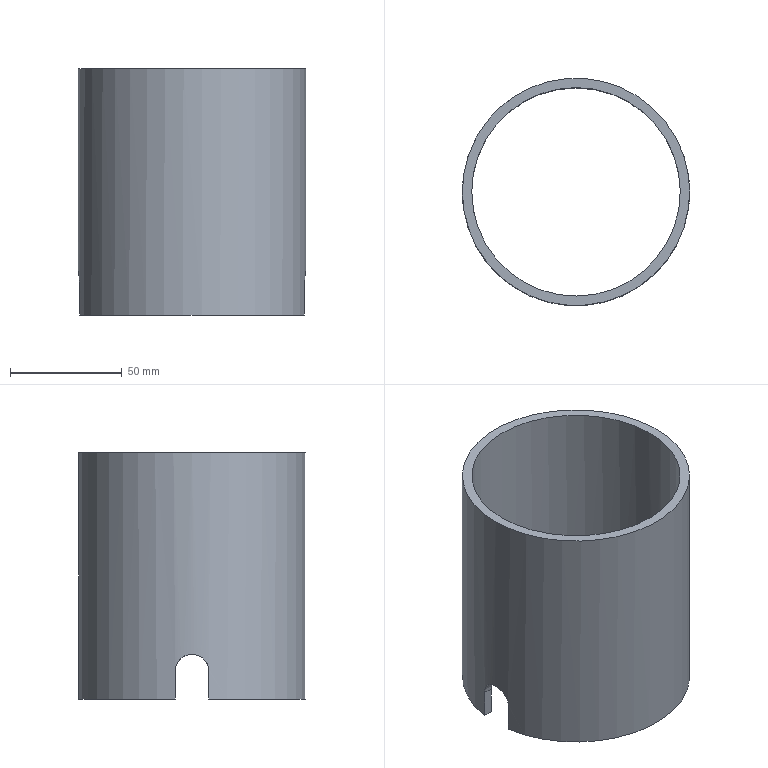Part | NX | features solid 2 | 1 solid | 11 faces | box 101.6 x 101.6 x 110 mm | volume 139042 mm3 | plane 7 | cylinder 4 | commonest cylinder face diameters 15 x2 93.2 x1 101.6 x1
STEP:
#1=CARTESIAN_POINT('',(-1250.243,532.5,-195.));
#2=VERTEX_POINT('',#1);
#3=CARTESIAN_POINT('',(-1245.992,532.5,-195.));
#4=VERTEX_POINT('',#3);
#5=CARTESIAN_POINT('',(-1200.,532.5,-195.));
#6=DIRECTION('',(1.,0.,0.));
#7=VECTOR('',#6,1000.);
#8=LINE('',#5,#7);
#9=EDGE_CURVE('',#2,#4,#8,.T.);
#10=ORIENTED_EDGE('',*,*,#9,.F.);
#11=CARTESIAN_POINT('',(-1149.757,532.5,-195.));
#12=VERTEX_POINT('',#11);
#13=CARTESIAN_POINT('',(-1200.,525.,-195.));
#14=DIRECTION('',(0.,0.,1.));
#15=DIRECTION('',(-1.,0.,0.));
#16=AXIS2_PLACEMENT_3D('',#13,#14,#15);
#17=CIRCLE('',#16,50.8);
#18=EDGE_CURVE('',#12,#2,#17,.T.);
#19=ORIENTED_EDGE('',*,*,#18,.F.);
#20=CARTESIAN_POINT('',(-1154.008,532.5,-195.));
#21=VERTEX_POINT('',#20);
#22=CARTESIAN_POINT('',(-1130.25,532.5,-195.));
#23=DIRECTION('',(-1.,0.,0.));
#24=VECTOR('',#23,1000.);
#25=LINE('',#22,#24);
#26=EDGE_CURVE('',#12,#21,#25,.T.);
#27=ORIENTED_EDGE('',*,*,#26,.T.);
#28=CARTESIAN_POINT('',(-1200.,525.,-195.));
#29=DIRECTION('',(0.,0.,1.));
#30=DIRECTION('',(-1.,0.,0.));
#31=AXIS2_PLACEMENT_3D('',#28,#29,#30);
#32=CIRCLE('',#31,46.6);
#33=EDGE_CURVE('',#21,#4,#32,.T.);
#34=ORIENTED_EDGE('',*,*,#33,.T.);
#35=EDGE_LOOP('',(#10,#19,#27,#34));
#36=FACE_BOUND('',#35,.T.);
#37=CARTESIAN_POINT('',(-1200.,525.,-195.));
#38=DIRECTION('',(0.,0.,1.));
#39=DIRECTION('',(-1.,0.,0.));
#40=AXIS2_PLACEMENT_3D('',#37,#38,#39);
#41=PLANE('',#40);
#42=ADVANCED_FACE('',(#36),#41,.F.);
#43=CARTESIAN_POINT('',(-1250.243,517.5,-195.));
#44=VERTEX_POINT('',#43);
#45=CARTESIAN_POINT('',(-1149.757,517.5,-195.));
#46=VERTEX_POINT('',#45);
#47=CARTESIAN_POINT('',(-1200.,525.,-195.));
#48=DIRECTION('',(0.,0.,1.));
#49=DIRECTION('',(-1.,0.,0.));
#50=AXIS2_PLACEMENT_3D('',#47,#48,#49);
#51=CIRCLE('',#50,50.8);
#52=EDGE_CURVE('',#44,#46,#51,.T.);
#53=ORIENTED_EDGE('',*,*,#52,.T.);
#54=CARTESIAN_POINT('',(-1149.757,517.5,-182.5));
#55=VERTEX_POINT('',#54);
#56=CARTESIAN_POINT('',(-1149.757,517.5,-195.));
#57=DIRECTION('',(0.,0.,-1.));
#58=VECTOR('',#57,1000.);
#59=LINE('',#56,#58);
#60=EDGE_CURVE('',#46,#55,#59,.F.);
#61=ORIENTED_EDGE('',*,*,#60,.T.);
#62=CARTESIAN_POINT('',(-1149.757,532.5,-182.5));
#63=VERTEX_POINT('',#62);
#64=CARTESIAN_POINT('',(-1149.757,517.5,-182.5));
#65=CARTESIAN_POINT('',(-1149.757,517.5,-180.54));
#66=CARTESIAN_POINT('',(-1149.477,519.114,-176.63));
#67=CARTESIAN_POINT('',(-1149.061,525.012,-174.184));
#68=CARTESIAN_POINT('',(-1149.477,530.875,-176.636));
#69=CARTESIAN_POINT('',(-1149.757,532.5,-180.518));
#70=CARTESIAN_POINT('',(-1149.757,532.5,-182.5));
#71=B_SPLINE_CURVE_WITH_KNOTS('',3,(#64,#65,#66,#67,#68,#69,#70),.UNSPECIFIED.,.F.,.F.,(4,1,1,1,4),(0.03597,0.04184,0.04771,0.05358,0.05945),.UNSPECIFIED.);
#72=EDGE_CURVE('',#55,#63,#71,.T.);
#73=ORIENTED_EDGE('',*,*,#72,.T.);
#74=CARTESIAN_POINT('',(-1149.757,532.5,-135.));
#75=DIRECTION('',(0.,0.,-1.));
#76=VECTOR('',#75,1000.);
#77=LINE('',#74,#76);
#78=EDGE_CURVE('',#12,#63,#77,.F.);
#79=ORIENTED_EDGE('',*,*,#78,.F.);
#80=ORIENTED_EDGE('',*,*,#18,.T.);
#81=CARTESIAN_POINT('',(-1250.243,532.5,-182.5));
#82=VERTEX_POINT('',#81);
#83=CARTESIAN_POINT('',(-1250.243,532.5,-135.));
#84=DIRECTION('',(0.,0.,-1.));
#85=VECTOR('',#84,1000.);
#86=LINE('',#83,#85);
#87=EDGE_CURVE('',#82,#2,#86,.T.);
#88=ORIENTED_EDGE('',*,*,#87,.F.);
#89=CARTESIAN_POINT('',(-1250.243,517.5,-182.5));
#90=VERTEX_POINT('',#89);
#91=CARTESIAN_POINT('',(-1250.243,532.5,-182.5));
#92=CARTESIAN_POINT('',(-1250.243,532.5,-180.54));
#93=CARTESIAN_POINT('',(-1250.523,530.886,-176.63));
#94=CARTESIAN_POINT('',(-1250.939,524.988,-174.184));
#95=CARTESIAN_POINT('',(-1250.523,519.125,-176.636));
#96=CARTESIAN_POINT('',(-1250.243,517.5,-180.518));
#97=CARTESIAN_POINT('',(-1250.243,517.5,-182.5));
#98=B_SPLINE_CURVE_WITH_KNOTS('',3,(#91,#92,#93,#94,#95,#96,#97),.UNSPECIFIED.,.F.,.F.,(4,1,1,1,4),(0.03597,0.04184,0.04771,0.05358,0.05945),.UNSPECIFIED.);
#99=EDGE_CURVE('',#82,#90,#98,.T.);
#100=ORIENTED_EDGE('',*,*,#99,.T.);
#101=CARTESIAN_POINT('',(-1250.243,517.5,-135.));
#102=DIRECTION('',(0.,0.,-1.));
#103=VECTOR('',#102,1000.);
#104=LINE('',#101,#103);
#105=EDGE_CURVE('',#90,#44,#104,.T.);
#106=ORIENTED_EDGE('',*,*,#105,.T.);
#107=EDGE_LOOP('',(#53,#61,#73,#79,#80,#88,#100,#106));
#108=FACE_BOUND('',#107,.T.);
#109=CARTESIAN_POINT('',(-1250.8,525.,-85.));
#110=VERTEX_POINT('',#109);
#111=CARTESIAN_POINT('',(-1200.,525.,-85.));
#112=DIRECTION('',(0.,0.,1.));
#113=DIRECTION('',(-1.,0.,0.));
#114=AXIS2_PLACEMENT_3D('',#111,#112,#113);
#115=CIRCLE('',#114,50.8);
#116=EDGE_CURVE('',#110,#110,#115,.T.);
#117=ORIENTED_EDGE('',*,*,#116,.F.);
#118=EDGE_LOOP('',(#117));
#119=FACE_BOUND('',#118,.T.);
#120=CARTESIAN_POINT('',(-1200.,525.,-135.));
#121=DIRECTION('',(0.,0.,-1.));
#122=DIRECTION('',(1.,0.,0.));
#123=AXIS2_PLACEMENT_3D('',#120,#121,#122);
#124=CYLINDRICAL_SURFACE('',#123,50.8);
#125=ADVANCED_FACE('',(#108,#119),#124,.T.);
#126=CARTESIAN_POINT('',(-1154.008,517.5,-195.));
#127=VERTEX_POINT('',#126);
#128=CARTESIAN_POINT('',(-1154.008,517.5,-182.5));
#129=VERTEX_POINT('',#128);
#130=CARTESIAN_POINT('',(-1154.008,517.5,-135.));
#131=DIRECTION('',(0.,0.,-1.));
#132=VECTOR('',#131,1000.);
#133=LINE('',#130,#132);
#134=EDGE_CURVE('',#127,#129,#133,.F.);
#135=ORIENTED_EDGE('',*,*,#134,.F.);
#136=CARTESIAN_POINT('',(-1245.992,517.5,-195.));
#137=VERTEX_POINT('',#136);
#138=CARTESIAN_POINT('',(-1200.,525.,-195.));
#139=DIRECTION('',(0.,0.,1.));
#140=DIRECTION('',(-1.,0.,0.));
#141=AXIS2_PLACEMENT_3D('',#138,#139,#140);
#142=CIRCLE('',#141,46.6);
#143=EDGE_CURVE('',#137,#127,#142,.T.);
#144=ORIENTED_EDGE('',*,*,#143,.F.);
#145=CARTESIAN_POINT('',(-1245.992,517.5,-182.5));
#146=VERTEX_POINT('',#145);
#147=CARTESIAN_POINT('',(-1245.992,517.5,-135.));
#148=DIRECTION('',(0.,0.,-1.));
#149=VECTOR('',#148,1000.);
#150=LINE('',#147,#149);
#151=EDGE_CURVE('',#146,#137,#150,.T.);
#152=ORIENTED_EDGE('',*,*,#151,.F.);
#153=CARTESIAN_POINT('',(-1245.992,532.5,-182.5));
#154=VERTEX_POINT('',#153);
#155=CARTESIAN_POINT('',(-1245.992,532.5,-182.5));
#156=CARTESIAN_POINT('',(-1245.992,532.5,-180.542));
#157=CARTESIAN_POINT('',(-1246.298,530.886,-176.629));
#158=CARTESIAN_POINT('',(-1246.751,524.99,-174.184));
#159=CARTESIAN_POINT('',(-1246.298,519.126,-176.633));
#160=CARTESIAN_POINT('',(-1245.992,517.5,-180.52));
#161=CARTESIAN_POINT('',(-1245.992,517.5,-182.5));
#162=B_SPLINE_CURVE_WITH_KNOTS('',3,(#155,#156,#157,#158,#159,#160,#161),.UNSPECIFIED.,.F.,.F.,(4,1,1,1,4),(0.03615,0.04202,0.04789,0.05376,0.05963),.UNSPECIFIED.);
#163=EDGE_CURVE('',#154,#146,#162,.T.);
#164=ORIENTED_EDGE('',*,*,#163,.F.);
#165=CARTESIAN_POINT('',(-1245.992,532.5,-135.));
#166=DIRECTION('',(0.,0.,-1.));
#167=VECTOR('',#166,1000.);
#168=LINE('',#165,#167);
#169=EDGE_CURVE('',#154,#4,#168,.T.);
#170=ORIENTED_EDGE('',*,*,#169,.T.);
#171=ORIENTED_EDGE('',*,*,#33,.F.);
#172=CARTESIAN_POINT('',(-1154.008,532.5,-182.5));
#173=VERTEX_POINT('',#172);
#174=CARTESIAN_POINT('',(-1154.008,532.5,-135.));
#175=DIRECTION('',(0.,0.,-1.));
#176=VECTOR('',#175,1000.);
#177=LINE('',#174,#176);
#178=EDGE_CURVE('',#21,#173,#177,.F.);
#179=ORIENTED_EDGE('',*,*,#178,.T.);
#180=CARTESIAN_POINT('',(-1154.008,517.5,-182.5));
#181=CARTESIAN_POINT('',(-1154.008,517.5,-180.542));
#182=CARTESIAN_POINT('',(-1153.702,519.114,-176.629));
#183=CARTESIAN_POINT('',(-1153.249,525.01,-174.184));
#184=CARTESIAN_POINT('',(-1153.702,530.874,-176.633));
#185=CARTESIAN_POINT('',(-1154.008,532.5,-180.52));
#186=CARTESIAN_POINT('',(-1154.008,532.5,-182.5));
#187=B_SPLINE_CURVE_WITH_KNOTS('',3,(#180,#181,#182,#183,#184,#185,#186),.UNSPECIFIED.,.F.,.F.,(4,1,1,1,4),(0.03615,0.04202,0.04789,0.05376,0.05963),.UNSPECIFIED.);
#188=EDGE_CURVE('',#129,#173,#187,.T.);
#189=ORIENTED_EDGE('',*,*,#188,.F.);
#190=EDGE_LOOP('',(#135,#144,#152,#164,#170,#171,#179,#189));
#191=FACE_BOUND('',#190,.T.);
#192=CARTESIAN_POINT('',(-1246.6,525.,-85.));
#193=VERTEX_POINT('',#192);
#194=CARTESIAN_POINT('',(-1200.,525.,-85.));
#195=DIRECTION('',(0.,0.,1.));
#196=DIRECTION('',(-1.,0.,0.));
#197=AXIS2_PLACEMENT_3D('',#194,#195,#196);
#198=CIRCLE('',#197,46.6);
#199=EDGE_CURVE('',#193,#193,#198,.T.);
#200=ORIENTED_EDGE('',*,*,#199,.T.);
#201=EDGE_LOOP('',(#200));
#202=FACE_BOUND('',#201,.T.);
#203=CARTESIAN_POINT('',(-1200.,525.,-135.));
#204=DIRECTION('',(0.,0.,-1.));
#205=DIRECTION('',(1.,0.,0.));
#206=AXIS2_PLACEMENT_3D('',#203,#204,#205);
#207=CYLINDRICAL_SURFACE('',#206,46.6);
#208=ADVANCED_FACE('',(#191,#202),#207,.F.);
#209=ORIENTED_EDGE('',*,*,#116,.T.);
#210=EDGE_LOOP('',(#209));
#211=FACE_BOUND('',#210,.T.);
#212=ORIENTED_EDGE('',*,*,#199,.F.);
#213=EDGE_LOOP('',(#212));
#214=FACE_BOUND('',#213,.T.);
#215=CARTESIAN_POINT('',(-1200.,525.,-85.));
#216=DIRECTION('',(0.,0.,1.));
#217=DIRECTION('',(-1.,0.,0.));
#218=AXIS2_PLACEMENT_3D('',#215,#216,#217);
#219=PLANE('',#218);
#220=ADVANCED_FACE('',(#211,#214),#219,.T.);
#221=ORIENTED_EDGE('',*,*,#52,.F.);
#222=CARTESIAN_POINT('',(-1200.,517.5,-195.));
#223=DIRECTION('',(1.,0.,0.));
#224=VECTOR('',#223,1000.);
#225=LINE('',#222,#224);
#226=EDGE_CURVE('',#44,#137,#225,.T.);
#227=ORIENTED_EDGE('',*,*,#226,.T.);
#228=ORIENTED_EDGE('',*,*,#143,.T.);
#229=CARTESIAN_POINT('',(-1130.25,517.5,-195.));
#230=DIRECTION('',(-1.,0.,0.));
#231=VECTOR('',#230,1000.);
#232=LINE('',#229,#231);
#233=EDGE_CURVE('',#46,#127,#232,.T.);
#234=ORIENTED_EDGE('',*,*,#233,.F.);
#235=EDGE_LOOP('',(#221,#227,#228,#234));
#236=FACE_BOUND('',#235,.T.);
#237=CARTESIAN_POINT('',(-1200.,525.,-195.));
#238=DIRECTION('',(0.,0.,1.));
#239=DIRECTION('',(-1.,0.,0.));
#240=AXIS2_PLACEMENT_3D('',#237,#238,#239);
#241=PLANE('',#240);
#242=ADVANCED_FACE('',(#236),#241,.F.);
#243=ORIENTED_EDGE('',*,*,#78,.T.);
#244=CARTESIAN_POINT('',(-1130.25,532.5,-182.5));
#245=DIRECTION('',(-1.,0.,0.));
#246=VECTOR('',#245,1000.);
#247=LINE('',#244,#246);
#248=EDGE_CURVE('',#173,#63,#247,.F.);
#249=ORIENTED_EDGE('',*,*,#248,.F.);
#250=ORIENTED_EDGE('',*,*,#178,.F.);
#251=ORIENTED_EDGE('',*,*,#26,.F.);
#252=EDGE_LOOP('',(#243,#249,#250,#251));
#253=FACE_BOUND('',#252,.T.);
#254=CARTESIAN_POINT('',(-1130.25,532.5,-195.));
#255=DIRECTION('',(0.,-1.,0.));
#256=DIRECTION('',(0.,0.,1.));
#257=AXIS2_PLACEMENT_3D('',#254,#255,#256);
#258=PLANE('',#257);
#259=ADVANCED_FACE('',(#253),#258,.T.);
#260=ORIENTED_EDGE('',*,*,#233,.T.);
#261=ORIENTED_EDGE('',*,*,#134,.T.);
#262=CARTESIAN_POINT('',(-1330.25,517.5,-182.5));
#263=DIRECTION('',(-1.,0.,0.));
#264=VECTOR('',#263,1000.);
#265=LINE('',#262,#264);
#266=EDGE_CURVE('',#55,#129,#265,.T.);
#267=ORIENTED_EDGE('',*,*,#266,.F.);
#268=ORIENTED_EDGE('',*,*,#60,.F.);
#269=EDGE_LOOP('',(#260,#261,#267,#268));
#270=FACE_BOUND('',#269,.T.);
#271=CARTESIAN_POINT('',(-1130.25,517.5,-195.));
#272=DIRECTION('',(0.,-1.,0.));
#273=DIRECTION('',(0.,0.,1.));
#274=AXIS2_PLACEMENT_3D('',#271,#272,#273);
#275=PLANE('',#274);
#276=ADVANCED_FACE('',(#270),#275,.F.);
#277=ORIENTED_EDGE('',*,*,#266,.T.);
#278=ORIENTED_EDGE('',*,*,#188,.T.);
#279=ORIENTED_EDGE('',*,*,#248,.T.);
#280=ORIENTED_EDGE('',*,*,#72,.F.);
#281=EDGE_LOOP('',(#277,#278,#279,#280));
#282=FACE_BOUND('',#281,.T.);
#283=CARTESIAN_POINT('',(-1130.25,525.,-182.5));
#284=DIRECTION('',(1.,0.,0.));
#285=DIRECTION('',(0.,0.,1.));
#286=AXIS2_PLACEMENT_3D('',#283,#284,#285);
#287=CYLINDRICAL_SURFACE('',#286,7.5);
#288=ADVANCED_FACE('',(#282),#287,.F.);
#289=CARTESIAN_POINT('',(-1130.25,532.5,-182.5));
#290=DIRECTION('',(-1.,0.,0.));
#291=VECTOR('',#290,1000.);
#292=LINE('',#289,#291);
#293=EDGE_CURVE('',#82,#154,#292,.F.);
#294=ORIENTED_EDGE('',*,*,#293,.T.);
#295=ORIENTED_EDGE('',*,*,#163,.T.);
#296=CARTESIAN_POINT('',(-1330.25,517.5,-182.5));
#297=DIRECTION('',(-1.,0.,0.));
#298=VECTOR('',#297,1000.);
#299=LINE('',#296,#298);
#300=EDGE_CURVE('',#146,#90,#299,.T.);
#301=ORIENTED_EDGE('',*,*,#300,.T.);
#302=ORIENTED_EDGE('',*,*,#99,.F.);
#303=EDGE_LOOP('',(#294,#295,#301,#302));
#304=FACE_BOUND('',#303,.T.);
#305=CARTESIAN_POINT('',(-1130.25,525.,-182.5));
#306=DIRECTION('',(1.,0.,0.));
#307=DIRECTION('',(0.,0.,1.));
#308=AXIS2_PLACEMENT_3D('',#305,#306,#307);
#309=CYLINDRICAL_SURFACE('',#308,7.5);
#310=ADVANCED_FACE('',(#304),#309,.F.);
#311=ORIENTED_EDGE('',*,*,#300,.F.);
#312=ORIENTED_EDGE('',*,*,#151,.T.);
#313=ORIENTED_EDGE('',*,*,#226,.F.);
#314=ORIENTED_EDGE('',*,*,#105,.F.);
#315=EDGE_LOOP('',(#311,#312,#313,#314));
#316=FACE_BOUND('',#315,.T.);
#317=CARTESIAN_POINT('',(-1130.25,517.5,-195.));
#318=DIRECTION('',(0.,-1.,0.));
#319=DIRECTION('',(0.,0.,1.));
#320=AXIS2_PLACEMENT_3D('',#317,#318,#319);
#321=PLANE('',#320);
#322=ADVANCED_FACE('',(#316),#321,.F.);
#323=ORIENTED_EDGE('',*,*,#87,.T.);
#324=ORIENTED_EDGE('',*,*,#9,.T.);
#325=ORIENTED_EDGE('',*,*,#169,.F.);
#326=ORIENTED_EDGE('',*,*,#293,.F.);
#327=EDGE_LOOP('',(#323,#324,#325,#326));
#328=FACE_BOUND('',#327,.T.);
#329=CARTESIAN_POINT('',(-1130.25,532.5,-195.));
#330=DIRECTION('',(0.,-1.,0.));
#331=DIRECTION('',(0.,0.,1.));
#332=AXIS2_PLACEMENT_3D('',#329,#330,#331);
#333=PLANE('',#332);
#334=ADVANCED_FACE('',(#328),#333,.T.);
#335=CLOSED_SHELL('',(#42,#125,#208,#220,#242,#259,#276,#288,#310,#322,#334));
#336=MANIFOLD_SOLID_BREP('',#335);
#337=(LENGTH_UNIT()NAMED_UNIT(*)SI_UNIT(.MILLI.,.METRE.));
#338=UNCERTAINTY_MEASURE_WITH_UNIT(LENGTH_MEASURE(0.0508),#337,'','');
#339=(NAMED_UNIT(*)PLANE_ANGLE_UNIT()SI_UNIT($,.RADIAN.));
#340=(NAMED_UNIT(*)SI_UNIT($,.STERADIAN.)SOLID_ANGLE_UNIT());
#341=(GEOMETRIC_REPRESENTATION_CONTEXT(3)GLOBAL_UNCERTAINTY_ASSIGNED_CONTEXT((#338))GLOBAL_UNIT_ASSIGNED_CONTEXT((#337,#339,#340))REPRESENTATION_CONTEXT('',''));
#342=ADVANCED_BREP_SHAPE_REPRESENTATION('',(#336),#341);